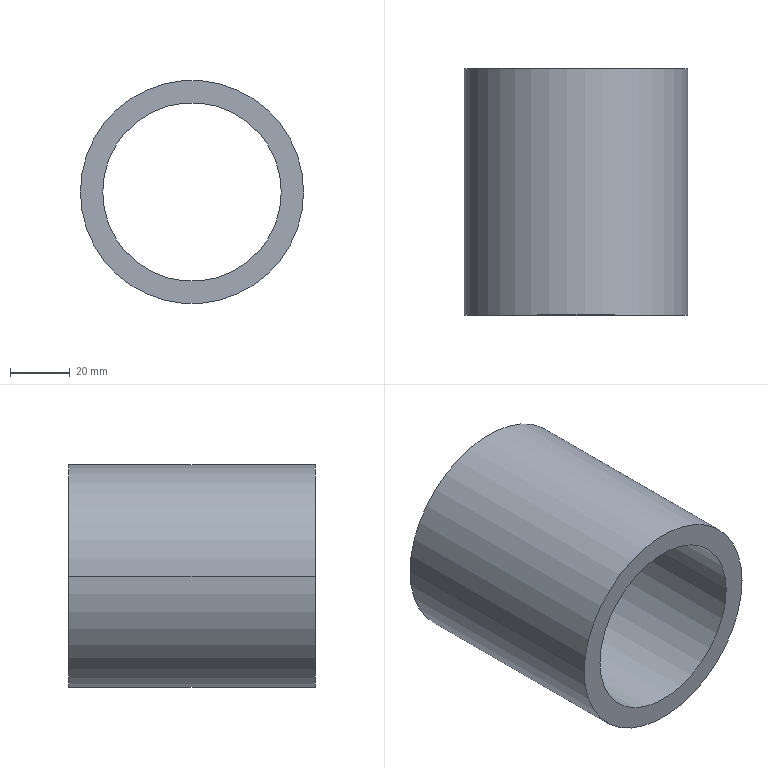Part | STEP file | Scale factor 1[10] | 1 solid | 6 faces | box 75 x 82.8 x 75 mm | volume 131688 mm3 | cylinder 4 | plane 2 | commonest cylinder face diameters 60 x2 75 x2
STEP:
#1=CARTESIAN_POINT('',(-778.738,-280.973,3238.5));
#2=VERTEX_POINT('',#1);
#3=CARTESIAN_POINT('',(-718.738,-280.973,3238.5));
#4=VERTEX_POINT('',#3);
#5=CARTESIAN_POINT('',(-748.738,-280.973,3238.5));
#6=DIRECTION('',(0.,1.,0.));
#7=DIRECTION('',(1.,0.,0.000000001));
#8=AXIS2_PLACEMENT_3D('',#5,#6,#7);
#9=CIRCLE('',#8,30.);
#10=EDGE_CURVE('',#2,#4,#9,.T.);
#11=ORIENTED_EDGE('',*,*,#10,.T.);
#12=CARTESIAN_POINT('',(-718.738,-363.773,3238.5));
#13=VERTEX_POINT('',#12);
#14=CARTESIAN_POINT('',(-718.738,-280.973,3238.5));
#15=DIRECTION('',(0.,1.,0.));
#16=VECTOR('',#15,1000.);
#17=LINE('',#14,#16);
#18=EDGE_CURVE('',#13,#4,#17,.T.);
#19=ORIENTED_EDGE('',*,*,#18,.F.);
#20=CARTESIAN_POINT('',(-778.738,-363.773,3238.5));
#21=VERTEX_POINT('',#20);
#22=CARTESIAN_POINT('',(-748.738,-363.773,3238.5));
#23=DIRECTION('',(0.,1.,0.));
#24=DIRECTION('',(1.,0.,0.000000001));
#25=AXIS2_PLACEMENT_3D('',#22,#23,#24);
#26=CIRCLE('',#25,30.);
#27=EDGE_CURVE('',#21,#13,#26,.T.);
#28=ORIENTED_EDGE('',*,*,#27,.F.);
#29=CARTESIAN_POINT('',(-778.738,-280.973,3238.5));
#30=DIRECTION('',(0.,1.,0.));
#31=VECTOR('',#30,1000.);
#32=LINE('',#29,#31);
#33=EDGE_CURVE('',#21,#2,#32,.T.);
#34=ORIENTED_EDGE('',*,*,#33,.T.);
#35=EDGE_LOOP('',(#11,#19,#28,#34));
#36=FACE_OUTER_BOUND('',#35,.T.);
#37=CARTESIAN_POINT('',(-748.738,-280.973,3238.5));
#38=DIRECTION('',(0.,-1.,0.));
#39=DIRECTION('',(1.,0.,0.000000001));
#40=AXIS2_PLACEMENT_3D('',#37,#38,#39);
#41=CYLINDRICAL_SURFACE('',#40,30.);
#42=ADVANCED_FACE('',(#36),#41,.F.);
#43=CARTESIAN_POINT('',(-711.238,-280.973,3238.5));
#44=VERTEX_POINT('',#43);
#45=CARTESIAN_POINT('',(-786.238,-280.973,3238.5));
#46=VERTEX_POINT('',#45);
#47=CARTESIAN_POINT('',(-748.738,-280.973,3238.5));
#48=DIRECTION('',(0.,1.,0.));
#49=DIRECTION('',(1.,0.,0.000000001));
#50=AXIS2_PLACEMENT_3D('',#47,#48,#49);
#51=CIRCLE('',#50,37.5);
#52=EDGE_CURVE('',#44,#46,#51,.T.);
#53=ORIENTED_EDGE('',*,*,#52,.F.);
#54=CARTESIAN_POINT('',(-711.238,-363.773,3238.5));
#55=VERTEX_POINT('',#54);
#56=CARTESIAN_POINT('',(-711.238,-280.973,3238.5));
#57=DIRECTION('',(0.,1.,0.));
#58=VECTOR('',#57,1000.);
#59=LINE('',#56,#58);
#60=EDGE_CURVE('',#55,#44,#59,.T.);
#61=ORIENTED_EDGE('',*,*,#60,.F.);
#62=CARTESIAN_POINT('',(-786.238,-363.773,3238.5));
#63=VERTEX_POINT('',#62);
#64=CARTESIAN_POINT('',(-748.738,-363.773,3238.5));
#65=DIRECTION('',(0.,1.,0.));
#66=DIRECTION('',(1.,0.,0.000000001));
#67=AXIS2_PLACEMENT_3D('',#64,#65,#66);
#68=CIRCLE('',#67,37.5);
#69=EDGE_CURVE('',#55,#63,#68,.T.);
#70=ORIENTED_EDGE('',*,*,#69,.T.);
#71=CARTESIAN_POINT('',(-786.238,-280.973,3238.5));
#72=DIRECTION('',(0.,1.,0.));
#73=VECTOR('',#72,1000.);
#74=LINE('',#71,#73);
#75=EDGE_CURVE('',#63,#46,#74,.T.);
#76=ORIENTED_EDGE('',*,*,#75,.T.);
#77=EDGE_LOOP('',(#53,#61,#70,#76));
#78=FACE_OUTER_BOUND('',#77,.T.);
#79=CARTESIAN_POINT('',(-748.738,-280.973,3238.5));
#80=DIRECTION('',(0.,-1.,0.));
#81=DIRECTION('',(1.,0.,0.000000001));
#82=AXIS2_PLACEMENT_3D('',#79,#80,#81);
#83=CYLINDRICAL_SURFACE('',#82,37.5);
#84=ADVANCED_FACE('',(#78),#83,.T.);
#85=CARTESIAN_POINT('',(-748.738,-280.973,3238.5));
#86=DIRECTION('',(0.,1.,0.));
#87=DIRECTION('',(1.,0.,0.000000001));
#88=AXIS2_PLACEMENT_3D('',#85,#86,#87);
#89=CIRCLE('',#88,37.5);
#90=EDGE_CURVE('',#46,#44,#89,.T.);
#91=ORIENTED_EDGE('',*,*,#90,.T.);
#92=ORIENTED_EDGE('',*,*,#52,.T.);
#93=EDGE_LOOP('',(#91,#92));
#94=FACE_OUTER_BOUND('',#93,.T.);
#95=ORIENTED_EDGE('',*,*,#10,.F.);
#96=CARTESIAN_POINT('',(-748.738,-280.973,3238.5));
#97=DIRECTION('',(0.,1.,0.));
#98=DIRECTION('',(1.,0.,0.000000001));
#99=AXIS2_PLACEMENT_3D('',#96,#97,#98);
#100=CIRCLE('',#99,30.);
#101=EDGE_CURVE('',#4,#2,#100,.T.);
#102=ORIENTED_EDGE('',*,*,#101,.F.);
#103=EDGE_LOOP('',(#95,#102));
#104=FACE_BOUND('',#103,.T.);
#105=CARTESIAN_POINT('',(-748.738,-280.973,3238.5));
#106=DIRECTION('',(0.,1.,0.));
#107=DIRECTION('',(-1.,0.,-0.000000001));
#108=AXIS2_PLACEMENT_3D('',#105,#106,#107);
#109=PLANE('',#108);
#110=ADVANCED_FACE('',(#94,#104),#109,.T.);
#111=CARTESIAN_POINT('',(-748.738,-363.773,3238.5));
#112=DIRECTION('',(0.,1.,0.));
#113=DIRECTION('',(1.,0.,0.000000001));
#114=AXIS2_PLACEMENT_3D('',#111,#112,#113);
#115=CIRCLE('',#114,37.5);
#116=EDGE_CURVE('',#63,#55,#115,.T.);
#117=ORIENTED_EDGE('',*,*,#116,.F.);
#118=ORIENTED_EDGE('',*,*,#69,.F.);
#119=EDGE_LOOP('',(#117,#118));
#120=FACE_OUTER_BOUND('',#119,.T.);
#121=ORIENTED_EDGE('',*,*,#27,.T.);
#122=CARTESIAN_POINT('',(-748.738,-363.773,3238.5));
#123=DIRECTION('',(0.,1.,0.));
#124=DIRECTION('',(1.,0.,0.000000001));
#125=AXIS2_PLACEMENT_3D('',#122,#123,#124);
#126=CIRCLE('',#125,30.);
#127=EDGE_CURVE('',#13,#21,#126,.T.);
#128=ORIENTED_EDGE('',*,*,#127,.T.);
#129=EDGE_LOOP('',(#121,#128));
#130=FACE_BOUND('',#129,.T.);
#131=CARTESIAN_POINT('',(-748.738,-363.773,3238.5));
#132=DIRECTION('',(0.,1.,0.));
#133=DIRECTION('',(-1.,0.,-0.000000001));
#134=AXIS2_PLACEMENT_3D('',#131,#132,#133);
#135=PLANE('',#134);
#136=ADVANCED_FACE('',(#120,#130),#135,.F.);
#137=ORIENTED_EDGE('',*,*,#60,.T.);
#138=ORIENTED_EDGE('',*,*,#90,.F.);
#139=ORIENTED_EDGE('',*,*,#75,.F.);
#140=ORIENTED_EDGE('',*,*,#116,.T.);
#141=EDGE_LOOP('',(#137,#138,#139,#140));
#142=FACE_OUTER_BOUND('',#141,.T.);
#143=CARTESIAN_POINT('',(-748.738,-280.973,3238.5));
#144=DIRECTION('',(0.,-1.,0.));
#145=DIRECTION('',(1.,0.,0.000000001));
#146=AXIS2_PLACEMENT_3D('',#143,#144,#145);
#147=CYLINDRICAL_SURFACE('',#146,37.5);
#148=ADVANCED_FACE('',(#142),#147,.T.);
#149=ORIENTED_EDGE('',*,*,#18,.T.);
#150=ORIENTED_EDGE('',*,*,#101,.T.);
#151=ORIENTED_EDGE('',*,*,#33,.F.);
#152=ORIENTED_EDGE('',*,*,#127,.F.);
#153=EDGE_LOOP('',(#149,#150,#151,#152));
#154=FACE_OUTER_BOUND('',#153,.T.);
#155=CARTESIAN_POINT('',(-748.738,-280.973,3238.5));
#156=DIRECTION('',(0.,-1.,0.));
#157=DIRECTION('',(1.,0.,0.000000001));
#158=AXIS2_PLACEMENT_3D('',#155,#156,#157);
#159=CYLINDRICAL_SURFACE('',#158,30.);
#160=ADVANCED_FACE('',(#154),#159,.F.);
#161=CLOSED_SHELL('',(#42,#84,#110,#136,#148,#160));
#162=MANIFOLD_SOLID_BREP('',#161);
#163=CARTESIAN_POINT('',(0.,0.,0.));
#164=DIRECTION('',(0.,0.,1.));
#165=DIRECTION('',(1.,0.,0.));
#166=AXIS2_PLACEMENT_3D('',#163,#164,#165);
#167=(LENGTH_UNIT()NAMED_UNIT(*)SI_UNIT(.MILLI.,.METRE.));
#168=UNCERTAINTY_MEASURE_WITH_UNIT(LENGTH_MEASURE(0.00001),#167,'','');
#169=(NAMED_UNIT(*)PLANE_ANGLE_UNIT()SI_UNIT($,.RADIAN.));
#170=(NAMED_UNIT(*)SI_UNIT($,.STERADIAN.)SOLID_ANGLE_UNIT());
#171=(GEOMETRIC_REPRESENTATION_CONTEXT(3)GLOBAL_UNCERTAINTY_ASSIGNED_CONTEXT((#168))GLOBAL_UNIT_ASSIGNED_CONTEXT((#167,#169,#170))REPRESENTATION_CONTEXT('',''));
#172=ADVANCED_BREP_SHAPE_REPRESENTATION('',(#162,#166),#171);